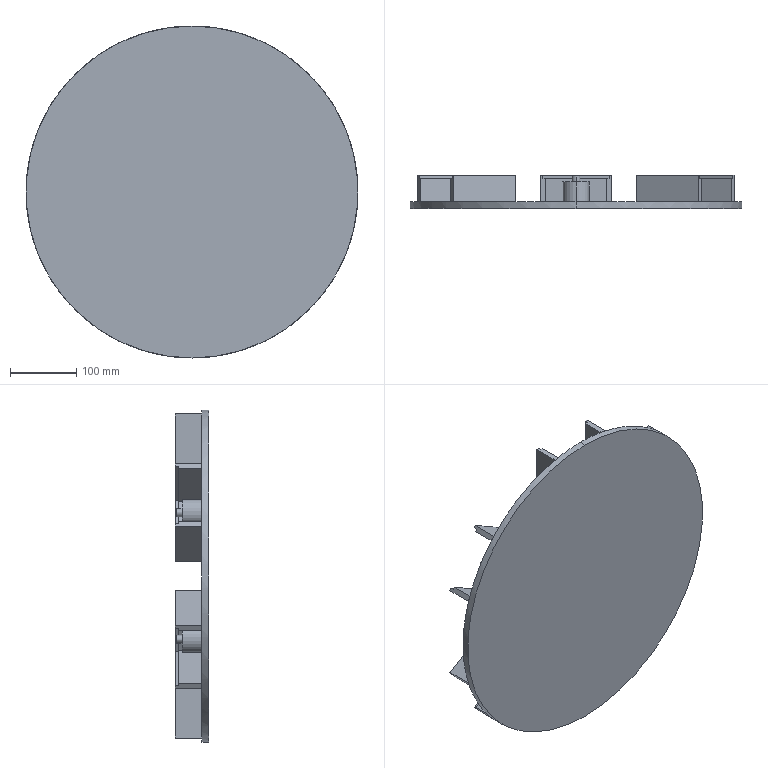Part | STEP file | Guide wheel mechanism revised.sldasm-Part-337 | 1 solid | 130 faces | box 500 x 50 x 500 mm | volume 2751729 mm3 | plane 92 | cylinder 26 | cone 12 | commonest cylinder face diameters 12 x12 40 x12 500 x2